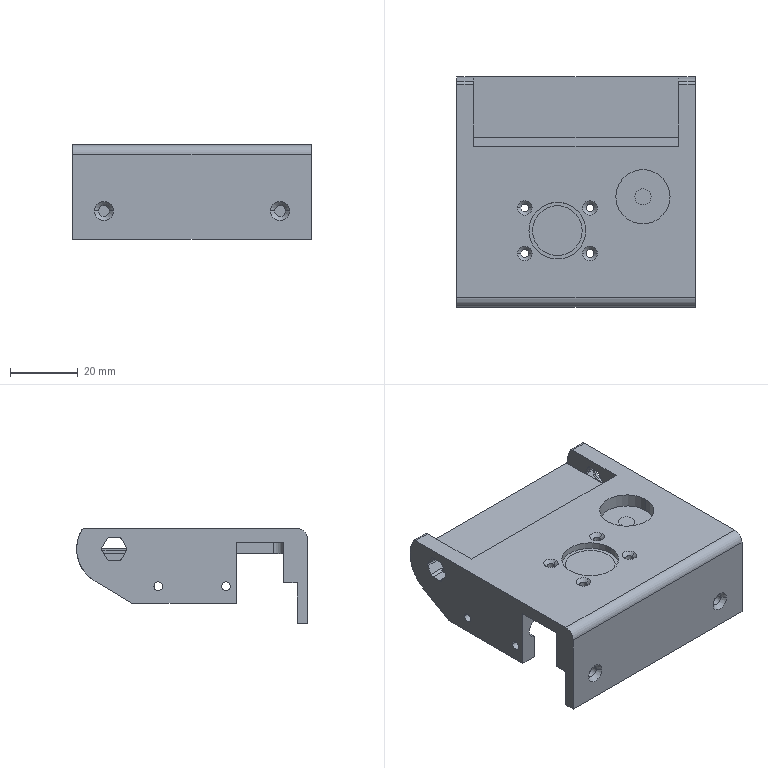NC program | NX | posted with a generic post | part box 70.5 x 68.1 x 28 mm
Lines 81 to 1012 of 7250:
(FLOOR_WALL_2 , TOOL : D10)
N160 T10 M6
N162 G54
N164 G17 G0 G90 X73.15 Y-43.397 B0. C0. S9500 M3
N166 G43 Z30. H10
N168 Z-2.85
N170 G94 G1 Z-5.85 F1000.
N172 Y-40.397
N174 Y40.397 F3000.
N176 X72.15
N178 Y-40.397
N180 X71.15
N182 Y40.397
N184 X70.15
N186 Y-40.397
N188 X69.15
N190 Y40.397
N192 X68.15
N194 Y-40.397
N196 X67.15
N198 Y40.397
N200 X66.644
N202 X66.15
N204 Y-40.397
N206 X65.776
N208 X65.15
N210 Y40.397
N212 X64.15
N214 Y-40.397
N216 X63.15
N218 Y40.397
N220 X62.15
N222 Y-40.397
N224 X61.15
N226 Y40.397
N228 X60.15
N230 Y-40.397
N232 X59.15
N234 Y40.397
N236 X58.15
N238 Y-40.397
N240 X57.15
N242 Y40.397
N244 X56.15
N246 Y-40.397
N248 X55.15
N250 Y40.397
N252 X54.15
N254 Y-40.397
N256 X53.15
N258 Y40.397
N260 X52.15
N262 Y-40.397
N264 X51.15
N266 Y40.397
N268 X50.15
N270 Y-40.397
N272 X49.15
N274 Y40.397
N276 X48.15
N278 Y-40.397
N280 X47.15
N282 Y40.397
N284 X46.15
N286 Y-40.397
N288 X45.15
N290 Y40.397
N292 X44.15
N294 Y-40.397
N296 X43.15
N298 Y40.397
N300 X42.15
N302 Y-40.397
N304 X41.15
N306 Y40.397
N308 X40.15
N310 Y-40.397
N312 X39.15
N314 Y40.397
N316 X38.15
N318 Y-40.397
N320 X37.15
N322 Y40.397
N324 X36.15
N326 Y-40.397
N328 X35.15
N330 Y40.397
N332 X34.15
N334 Y-40.397
N336 X33.15
N338 Y40.397
N340 X32.15
N342 Y-40.397
N344 X31.15
N346 Y40.397
N348 X30.15
N350 Y-40.397
N352 X29.15
N354 Y40.397
N356 X28.15
N358 Y-40.397
N360 X27.15
N362 Y40.397
N364 X26.15
N366 Y-40.397
N368 X25.15
N370 Y40.397
N372 X24.15
N374 Y-40.397
N376 X23.15
N378 Y40.397
N380 X22.15
N382 Y-40.397
N384 X21.15
N386 Y40.397
N388 X20.15
N390 Y-40.397
N392 X19.15
N394 Y40.397
N396 X18.15
N398 Y-40.397
N400 X17.15
N402 Y40.397
N404 X16.15
N406 Y-40.397
N408 X15.15
N410 Y40.397
N412 X14.15
N414 Y-40.397
N416 X13.15
N418 Y40.397
N420 X12.15
N422 Y-40.397
N424 X11.15
N426 Y40.397
N428 X10.15
N430 Y-40.397
N432 X9.15
N434 Y40.397
N436 X8.15
N438 Y-40.397
N440 Y-43.4
N442 Z-2.85
N444 G0 Z30.
(ADAPTIVE_MILLING_COPY , TOOL : D10)
N446 X14.586 Y-41.708
N448 Z-20.85
N450 G1 Z-23.85 F1000.
N452 G3 X16. Y-40.294 R2.03 F3000.
N454 X12.857 Y-39.655 R6.057
N456 X12.02 Y-40.252 R1.803
N458 G1 Y-40.377
N460 G3 X13.172 Y-41.477 R1.104
N462 G1 X14.952 Y-41.392
N464 G3 X16. Y-40.294 R1.104
N466 X12.824 Y-39.329 R3.152
N468 X12.02 Y-40.303 R1.124
N470 X13.127 Y-41.404 R1.104
N472 G1 X14.906 Y-41.394
N474 G3 X16. Y-40.294 R1.104
N476 X14.067 Y-38.886 R2.409
N478 X12.234 Y-39.414 R1.891
N480 X12.02 Y-40.244 R1.35
N482 X13.09 Y-41.345 R1.104
N484 G1 X14.87 Y-41.393
N486 G3 X16. Y-40.294 R1.104
N488 X14.831 Y-38.788 R1.871
N490 X12.354 Y-38.943 R2.282
N492 X12.02 Y-40.021 R1.337
N494 X13.03 Y-41.118 R1.106
N496 G1 X14.81 Y-41.265
N498 G3 X16. Y-40.169 R1.104
N500 X14.791 Y-38.428 R1.881
N502 X12.322 Y-38.639 R2.246
N504 X12.021 Y-39.688 R1.367
N506 X12.98 Y-40.78 R1.106
N508 G1 X14.759 Y-41.009
N510 G3 X16. Y-39.919 R1.103
N512 X14.64 Y-38.024 R1.947
N514 X12.296 Y-38.33 R2.171
N516 X12.021 Y-39.352 R1.396
N518 X12.929 Y-40.436 R1.106
N520 G1 X14.708 Y-40.752
N522 G3 X16. Y-39.669 R1.103
N524 X14.607 Y-37.672 R1.968
N526 X12.273 Y-38.022 R2.137
N528 X12.021 Y-39.01 R1.413
N530 X12.949 Y-40.098 R1.106
N532 G1 X14.728 Y-40.38
N534 G3 X16. Y-39.294 R1.103
N536 X14.686 Y-37.368 R1.939
N538 X12.33 Y-37.622 R2.228
N540 X12.022 Y-38.676 R1.359
N542 X12.9 Y-39.755 R1.106
N544 G1 X14.678 Y-40.121
N546 G3 X16. Y-39.044 R1.103
N548 X14.533 Y-36.972 R2.
N550 X12.302 Y-37.315 R2.164
N552 X12.022 Y-38.346 R1.394
N554 X12.926 Y-39.429 R1.106
N556 G1 X14.704 Y-39.751
N558 G3 X16. Y-38.669 R1.103
N560 X14.613 Y-36.666 R1.973
N562 X12.277 Y-37.01 R2.142
N564 X12.023 Y-38.004 R1.41
N566 X12.946 Y-39.091 R1.106
N568 G1 X14.724 Y-39.379
N570 G3 X16. Y-38.294 R1.103
N572 X14.691 Y-36.365 R1.939
N574 X12.334 Y-36.614 R2.227
N576 X12.023 Y-37.671 R1.355
N578 X12.972 Y-38.762 R1.106
N580 G1 X14.749 Y-39.008
N582 G3 X16. Y-37.919 R1.103
N584 X14.653 Y-36.013 R1.956
N586 X12.306 Y-36.309 R2.189
N588 X12.023 Y-37.343 R1.393
N590 X12.926 Y-38.427 R1.106
N592 G1 X14.703 Y-38.751
N594 G3 X16. Y-37.669 R1.103
N596 X14.616 Y-35.663 R1.974
N598 X12.28 Y-36.004 R2.143
N600 X12.024 Y-37.019 R1.328
N602 X12.956 Y-38.107 R1.106
N604 G1 X14.733 Y-38.381
N606 G3 X16. Y-37.294 R1.103
N608 X14.696 Y-35.359 R1.948
N610 X12.341 Y-35.61 R2.196
N612 X12.024 Y-36.594 R1.396
N614 X12.927 Y-37.678 R1.106
N616 G1 X14.703 Y-38.001
N618 G3 X16. Y-36.919 R1.103
N620 X14.52 Y-34.954 R1.997
N622 X12.398 Y-35.252 R2.083
N624 X12.052 Y-36.218 R1.725
N626 X13.01 Y-37.493 R1.104
N628 G1 X14.765 Y-37.695
N630 G3 X15.988 Y-36.52 R1.103
N632 X13.967 Y-34.496 R2.156
N634 X12.292 Y-35.092 R1.673
N636 X12.114 Y-35.848 R1.712
N638 X13.058 Y-37.06 R1.104
N640 G1 X13.951 Y-37.188
N642 X14.847 Y-37.29
N644 G3 X15.913 Y-36.025 R1.103
N646 X14.277 Y-34.228 R2.011
N648 X12.411 Y-34.625 R1.893
N650 X12.128 Y-35.639 R1.552
N652 X13.118 Y-36.795 R1.104
N654 G1 X13.98 Y-36.887
N656 X14.845 Y-36.953
N658 G3 X15.88 Y-35.794 R1.104
N660 X14.452 Y-33.961 R1.896
N662 X12.371 Y-34.362 R1.881
N664 X12.15 Y-35.235 R1.355
N666 X13.074 Y-36.321 R1.106
N668 G1 X14.585 Y-36.566
N670 G3 X15.859 Y-35.42 R1.103
N672 X14.449 Y-33.643 R1.877
N674 X12.369 Y-34.05 R1.878
N676 X12.15 Y-35.002 R1.461
N678 X13.081 Y-36.089 R1.106
N680 G1 X13.915 Y-36.225
N682 X14.753 Y-36.335
N684 G3 X15.85 Y-35.235 R1.104
N686 X14.515 Y-33.344 R1.851
N688 X12.412 Y-33.682 R1.973
N690 X12.15 Y-34.686 R1.403
N692 X13.123 Y-35.779 R1.106
N694 G1 X13.956 Y-35.881
N696 X14.792 Y-35.959
N698 G3 X15.85 Y-34.86 R1.104
N700 X14.457 Y-33.011 R1.854
N702 X12.375 Y-33.413 R1.893
N704 X12.15 Y-34.371 R1.45
N706 X13.077 Y-35.457 R1.106
N708 G1 X13.911 Y-35.597
N710 X14.749 Y-35.71
N712 G3 X15.85 Y-34.61 R1.104
N714 X14.519 Y-32.717 R1.848
N716 X12.416 Y-33.047 R1.97
N718 X12.15 Y-34.058 R1.4
N720 X13.121 Y-35.15 R1.106
N722 G1 X13.954 Y-35.254
N724 X14.789 Y-35.335
N726 G3 X15.85 Y-34.235 R1.104
N728 X14.464 Y-32.38 R1.859
N730 X12.379 Y-32.778 R1.91
N732 X12.15 Y-33.74 R1.442
N734 X13.073 Y-34.826 R1.106
N736 G1 X13.907 Y-34.969
N738 X14.745 Y-35.085
N740 G3 X15.85 Y-33.985 R1.104
N742 X14.406 Y-32.048 R1.874
N744 X12.42 Y-32.414 R1.948
N746 X12.15 Y-33.43 R1.398
N748 X13.119 Y-34.523 R1.106
N750 G1 X13.952 Y-34.628
N752 X14.788 Y-34.71
N754 G3 X15.85 Y-33.61 R1.104
N756 X14.473 Y-31.749 R1.852
N758 X12.385 Y-32.139 R1.923
N760 X12.15 Y-33.108 R1.433
N762 X13.068 Y-34.193 R1.106
N764 G1 X13.902 Y-34.34
N766 X14.741 Y-34.46
N768 G3 X15.85 Y-33.36 R1.104
N770 X14.413 Y-31.418 R1.874
N772 X12.425 Y-31.774 R1.949
N774 X12.15 Y-32.798 R1.395
N776 X13.114 Y-33.89 R1.106
N778 G1 X13.947 Y-34.
N780 X14.783 Y-34.085
N782 G3 X15.85 Y-32.985 R1.104
N784 X14.476 Y-31.121 R1.852
N786 X12.387 Y-31.503 R1.921
N788 X12.15 Y-32.461 R1.413
N790 X13.052 Y-33.543 R1.106
N792 G1 X13.887 Y-33.702
N794 X14.726 Y-33.835
N796 G3 X15.85 Y-32.735 R1.104
N798 X14.537 Y-30.829 R1.85
N800 X12.429 Y-31.135 R1.991
N802 X12.15 Y-32.165 R1.394
N804 X13.108 Y-33.256 R1.106
N806 G1 X13.942 Y-33.371
N808 X14.778 Y-33.46
N810 G3 X15.85 Y-32.36 R1.104
N812 X14.481 Y-30.493 R1.854
N814 X12.39 Y-30.867 R1.922
N816 X12.15 Y-31.826 R1.403
N818 X13.045 Y-32.907 R1.106
N820 G1 X14.545 Y-33.191
N822 G3 X15.85 Y-32.11 R1.103
N824 X14.428 Y-30.154 R1.88
N826 X12.434 Y-30.499 R1.983
N828 X12.15 Y-31.538 R1.392
N830 X13.107 Y-32.629 R1.106
N832 G1 X13.94 Y-32.744
N834 X14.776 Y-32.835
N836 G3 X15.85 Y-31.735 R1.104
N838 X14.488 Y-29.865 R1.845
N840 X12.395 Y-30.231 R1.932
N842 X12.15 Y-31.214 R1.419
N844 X13.054 Y-32.296 R1.106
N846 G1 X13.889 Y-32.454
N848 X14.728 Y-32.585
N850 G3 X15.85 Y-31.485 R1.104
N852 X14.435 Y-29.525 R1.88
N854 X12.361 Y-29.962 R1.886
N856 X12.15 Y-30.914 R1.49
N858 X13.107 Y-32.005 R1.106
N860 G1 X13.94 Y-32.12
N862 X14.777 Y-32.21
N864 G3 X15.85 Y-31.11 R1.104
N866 X14.497 Y-29.236 R1.832
N868 X12.402 Y-29.594 R1.942
N870 X12.15 Y-30.585 R1.412
N872 X13.14 Y-31.679 R1.106
N874 G1 X13.973 Y-31.768
N876 X14.807 Y-31.834
N878 G3 X15.85 Y-30.735 R1.104
N880 X14.441 Y-28.897 R1.858
N882 X12.364 Y-29.323 R1.885
N884 X12.15 Y-30.278 R1.484
N886 X13.099 Y-31.367 R1.106
N888 G1 X13.933 Y-31.489
N890 X14.77 Y-31.585
N892 G3 X15.85 Y-30.485 R1.104
N894 X14.601 Y-28.643 R1.816
N896 X12.392 Y-28.973 R1.963
N898 X12.15 Y-29.951 R1.423
N900 X13.163 Y-31.048 R1.106
N902 G1 X14.002 Y-31.12
N904 X14.844 Y-31.169
N906 G3 X15.855 Y-30.216 R1.106
N908 X14.904 Y-28.471 R1.683
N910 X12.448 Y-28.589 R2.111
N912 X12.15 Y-29.639 R1.374
N914 X13.119 Y-30.731 R1.106
N916 G1 X13.976 Y-30.84
N918 X14.837 Y-30.923
N920 G3 X15.887 Y-29.968 R1.106
N922 X14.879 Y-28.128 R1.75
N924 X12.429 Y-28.294 R2.088
N926 X12.15 Y-29.324 R1.394
N928 X13.077 Y-30.411 R1.106
N930 G1 X14.656 Y-30.662
N932 G3 X15.92 Y-29.72 R1.104
N934 X14.863 Y-27.785 R1.788
N936 X12.5 Y-27.899 R2.193
N938 X12.15 Y-28.997 R1.328
N940 X13.028 Y-30.074 R1.106
N942 G1 X14.64 Y-30.406
N944 G3 X15.952 Y-29.472 R1.104
N946 X14.847 Y-27.442 R1.833
N948 X12.487 Y-27.589 R2.184
N950 X12.15 Y-28.672 R1.334
N952 X13.064 Y-29.757 R1.106
N954 G1 X14.725 Y-30.041
N956 G3 X16.001 Y-29.1 R1.104
N958 X14.957 Y-27.164 R1.801
N960 X12.486 Y-27.265 R2.212
N962 X12.15 Y-28.347 R1.335
N964 X13.026 Y-29.424 R1.106
N966 G1 X13.958 Y-29.624
N968 X14.895 Y-29.8
N970 G3 X16.016 Y-28.986 R1.106
N972 X15.377 Y-27.097 R1.668
N974 X12.488 Y-26.934 R2.312
N976 X12.15 Y-28.018 R1.334
N978 X13.002 Y-29.09 R1.106
N980 G1 X14.788 Y-29.503
N982 G3 X16.052 Y-28.853 R1.106
N984 X15.607 Y-26.927 R1.622
N986 X12.521 Y-26.573 R2.403
N988 X12.15 Y-27.697 R1.323
N990 X12.966 Y-28.76 R1.108
N992 G1 X14.847 Y-29.263
N994 G3 X16.148 Y-28.622 R1.106
N996 X15.667 Y-26.587 R1.705
N998 X12.567 Y-26.197 R2.494
N1000 X12.15 Y-27.35 R1.288
N1002 X12.921 Y-28.399 R1.108
N1004 G1 X14.898 Y-29.019
N1006 G3 X16.243 Y-28.391 R1.106
N1008 X15.825 Y-26.335 R1.746
N1010 X12.625 Y-25.81 R2.605
N1012 X12.15 Y-27.018 R1.276
N1014 X12.889 Y-28.057 R1.108
N1016 G1 X14.962 Y-28.778
N1018 G3 X16.339 Y-28.16 R1.104
N1020 X15.909 Y-25.992 R1.816
N1022 X12.596 Y-25.484 R2.651
N1024 X12.15 Y-26.662 R1.278
N1026 X12.906 Y-27.707 R1.108
N1028 G1 X15.122 Y-28.437
N1030 G3 X16.483 Y-27.813 R1.106
N1032 X16.198 Y-25.876 R1.743
N1034 X12.616 Y-25.113 R2.768
N1036 X12.15 Y-26.31 R1.276
N1038 X12.859 Y-27.338 R1.108
N1040 G1 X15.169 Y-28.217
N1042 G3 X16.513 Y-27.739 R1.106
N1044 X16.517 Y-25.846 R1.647
N1046 X12.72 Y-24.685 R2.89
N1048 X12.15 Y-25.952 R1.256
N1050 X12.836 Y-26.971 R1.108
N1052 G1 X15.296 Y-27.969
N1054 G3 X16.582 Y-27.62 R1.108
N1056 X16.728 Y-25.641 R1.666
N1058 X12.768 Y-24.286 R3.016
N1060 X12.15 Y-25.698 R1.362
N1062 X12.838 Y-26.718 R1.108
N1064 G1 X15.45 Y-27.772
N1066 G3 X16.735 Y-27.421 R1.108
N1068 X16.894 Y-25.326 R1.768
N1070 X12.726 Y-23.931 R3.115
N1072 X12.15 Y-25.204 R1.259
N1074 X12.807 Y-26.211 R1.111
N1076 G1 X15.647 Y-27.461
N1078 G3 X16.963 Y-27.124 R1.107
N1080 X17.075 Y-25.013 R1.848
N1082 X12.809 Y-23.495 R3.266
N1084 X12.15 Y-24.938 R1.37
N1086 X12.806 Y-25.944 R1.111
N1088 G1 X15.799 Y-27.263
N1090 G3 X17.115 Y-26.926 R1.106
N1092 X17.294 Y-24.743 R1.923
N1094 X12.847 Y-23.081 R3.405
N1096 X12.15 Y-24.551 R1.376
N1098 X12.836 Y-25.57 R1.108
N1100 G1 X16.124 Y-26.905
N1102 G3 X17.316 Y-26.664 R1.108
N1104 X17.639 Y-24.784 R1.779
N1106 X12.972 Y-22.613 R3.57
N1108 X12.15 Y-24.138 R1.377
N1110 X12.803 Y-25.143 R1.111
N1112 G1 X16.297 Y-26.698
N1114 G3 X17.414 Y-26.566 R1.112
N1116 X17.958 Y-24.874 R1.664
N1118 X12.926 Y-22.216 R3.692
N1120 X12.15 Y-23.726 R1.382
N1122 X12.738 Y-24.699 R1.112
N1124 G1 X16.331 Y-26.591
N1126 G3 X17.513 Y-26.49 R1.111
N1128 X18.191 Y-24.49 R1.838
N1130 X12.915 Y-21.789 R3.872
N1132 X12.15 Y-23.296 R1.389
N1134 X12.704 Y-24.251 R1.112
N1136 G1 X16.495 Y-26.42
N1138 G3 X17.711 Y-26.338 R1.108
N1140 X18.487 Y-24.365 R1.891
N1142 X13.049 Y-21.286 R4.079
N1144 X12.15 Y-22.868 R1.414
N1146 X12.699 Y-23.819 R1.112
N1148 G1 X16.788 Y-26.189
N1150 G3 X18.009 Y-26.109 R1.108
N1152 X18.775 Y-24.122 R1.976
N1154 X13.096 Y-20.812 R4.284
N1156 X12.15 Y-22.411 R1.423
N1158 X12.668 Y-23.345 R1.113
N1160 G1 X16.955 Y-26.018
N1162 G3 X18.207 Y-25.957 R1.108
N1164 X19.081 Y-23.934 R2.035
N1166 X15.181 Y-20.104 R4.486
N1168 X12.473 Y-20.761 R3.339
N1170 X12.15 Y-21.955 R1.507
N1172 X12.657 Y-22.882 R1.113
N1174 G1 X17.227 Y-25.806
N1176 G3 X18.37 Y-25.832 R1.112
N1178 X19.402 Y-24.094 R1.866
N1180 X16.84 Y-20.106 R4.432
N1182 X12.874 Y-19.997 R4.281
N1184 X12.15 Y-21.49 R1.408
N1186 X12.634 Y-22.402 R1.115
N1188 G1 X17.452 Y-25.658
N1190 G3 X18.489 Y-25.763 R1.115
N1192 X19.703 Y-24.167 R1.811
N1194 X17.668 Y-20.003 R4.446
N1196 X13.043 Y-19.423 R4.702
N1198 X12.15 Y-21.021 R1.444
N1200 X12.623 Y-21.925 R1.116
N1202 G1 X17.788 Y-25.507
N1204 G3 X18.836 Y-25.62 R1.113
N1206 X20.047 Y-24.004 R1.93
N1208 X18.185 Y-19.742 R4.61
N1210 X13.135 Y-18.884 R5.003
N1212 X12.15 Y-20.527 R1.473
N1214 X12.597 Y-21.412 R1.116
N1216 G1 X17.993 Y-25.393
N1218 G3 X19.067 Y-25.524 R1.112
N1220 X20.422 Y-23.731 R2.078
N1222 X18.436 Y-19.26 R4.881
N1224 X13.264 Y-18.32 R5.295
N1226 X12.15 Y-19.535 R1.582
N1228 G1 Y-20.035
N1230 G3 X12.588 Y-20.913 R1.116
N1232 G1 X18.33 Y-25.243
N1234 G3 X19.413 Y-25.381 R1.112
N1236 X20.782 Y-23.638 R2.137
N1238 X19.13 Y-19.139 R4.974
N1240 X13.469 Y-17.721 R5.693
N1242 X12.227 Y-18.698 R2.008
N1244 X12.15 Y-19.643 R2.957
N1246 X12.586 Y-20.519 R1.116
N1248 G1 X18.654 Y-25.116
N1250 G3 X19.603 Y-25.302 R1.116
N1252 X21.056 Y-23.88 R1.957
N1254 X20.037 Y-19.317 R4.878
N1256 X13.796 Y-17.083 R6.142
N1258 X12.267 Y-18.086 R2.454
N1260 X12.15 Y-19.116 R2.365
N1262 X12.564 Y-19.976 R1.117
N1264 G1 X18.907 Y-25.036
N1266 G3 X19.736 Y-25.266 R1.128
N1268 X21.335 Y-24.037 R1.915
N1270 X20.837 Y-19.503 R4.832
N1272 X13.957 Y-16.494 R6.516
N1274 X12.289 Y-17.512 R2.715
N1276 X12.15 Y-18.595 R2.219
N1278 X12.542 Y-19.437 R1.117
N1280 G1 X19.132 Y-24.985
N1282 G3 X19.984 Y-25.234 R1.127
N1284 X21.773 Y-23.871 R2.087
N1286 X21.3 Y-19.204 R5.095
N1288 X14.042 Y-15.912 R6.861
N1290 X12.275 Y-16.998 R2.775
N1292 X12.15 Y-18.047 R2.299
N1294 X12.529 Y-18.877 R1.118
N1296 G1 X19.491 Y-24.925
N1298 G3 X20.356 Y-25.185 R1.118
N1300 X22.167 Y-23.836 R2.175
N1302 X21.907 Y-19.141 R5.247
N1304 X14.29 Y-15.285 R7.254
N1306 X12.345 Y-16.328 R3.361
N1308 X12.15 Y-17.497 R1.956
N1310 X12.517 Y-18.317 R1.118
N1312 G1 X19.851 Y-24.866
N1314 G3 X20.728 Y-25.136 R1.117
N1316 X22.594 Y-23.762 R2.256
N1318 X22.443 Y-18.936 R5.485
N1320 X14.398 Y-14.682 R7.607
N1322 X12.341 Y-15.772 R3.498
N1324 X12.15 Y-16.934 R1.965
N1326 X12.511 Y-17.749 R1.118
N1328 G1 X13.164 Y-18.342
N1330 X14.645 Y-19.686 Z-23.75
N1332 X18.398 Y-23.092
N1334 X19.879 Y-24.436 Z-23.85
N1336 X20.423 Y-24.914
N1338 G3 X21.035 Y-25.1 R1.15
N1340 X22.867 Y-23.983 R2.123
N1342 X23.165 Y-19.167 R5.428
N1344 X14.618 Y-14.047 R8.007
N1346 X12.331 Y-15.213 R3.637
N1348 X12.15 Y-16.357 R1.995
N1350 X12.492 Y-17.154 R1.127
N1352 G1 X13.196 Y-17.824
N1354 X14.646 Y-19.203 Z-23.75
N1356 X18.631 Y-22.994
N1358 X20.08 Y-24.372 Z-23.85
N1360 X20.656 Y-24.903
N1362 G3 X21.285 Y-25.1 R1.148
N1364 X23.268 Y-24.01 R2.215
N1366 X23.824 Y-19.325 R5.512
N1368 X14.763 Y-13.416 R8.404
N1370 X12.347 Y-14.603 R3.894
N1372 X12.15 Y-15.776 R1.952
N1374 X12.481 Y-16.563 R1.128
N1376 G1 X13.216 Y-17.281
N1378 X14.646 Y-18.68 Z-23.75
N1380 X18.947 Y-22.886
N1382 X20.377 Y-24.284 Z-23.85
N1384 X21.021 Y-24.896
N1386 G3 X21.66 Y-25.1 R1.146
N1388 X23.746 Y-23.949 R2.341
N1390 X24.378 Y-19.146 R5.748
N1392 X14.945 Y-12.772 R8.818
N1394 X12.387 Y-13.957 R4.237
N1396 X12.15 Y-15.178 R1.835
N1398 X12.471 Y-15.955 R1.128
N1400 G1 X13.235 Y-16.722
N1402 X14.646 Y-18.139 Z-23.75
N1404 X19.302 Y-22.815
N1406 X20.714 Y-24.232 Z-23.85
N1408 X21.044 Y-24.566
N1410 X21.387 Y-24.889
N1412 G3 X22.035 Y-25.1 R1.145
N1414 X24.158 Y-24.004 R2.415
N1416 X25.008 Y-19.228 R5.88
N1418 X15.041 Y-12.131 R9.232
N1420 X12.374 Y-13.369 R4.314
N1422 X12.15 Y-14.576 R1.867
N1424 X12.461 Y-15.343 R1.129
N1426 G1 X13.252 Y-16.157
N1428 X14.646 Y-17.591 Z-23.75
N1430 X19.672 Y-22.762
N1432 X21.066 Y-24.196 Z-23.85
N1434 X21.403 Y-24.546
N1436 X21.753 Y-24.883
N1438 G3 X22.41 Y-25.1 R1.144
N1440 X24.651 Y-23.972 R2.531
N1442 X25.566 Y-18.961 R6.187
N1444 X15.292 Y-11.46 R9.699
N1446 X12.382 Y-12.749 R4.591
N1448 X12.15 Y-13.965 R1.846
N1450 X12.453 Y-14.723 R1.13
N1452 G1 X13.269 Y-15.582
N1454 X14.647 Y-17.032 Z-23.75
N1456 X20.04 Y-22.708
N1458 X21.418 Y-24.158 Z-23.85
N1460 X21.762 Y-24.524
N1462 X22.12 Y-24.877
N1464 G3 X22.785 Y-25.1 R1.143
N1466 X25.147 Y-23.951 R2.625
N1468 X26.163 Y-18.833 R6.402
N1470 X15.454 Y-10.792 R10.153
N1472 X12.413 Y-12.093 R4.879
N1474 X12.15 Y-13.349 R1.787
N1476 X12.449 Y-14.104 R1.13
N1478 G1 X13.275 Y-14.98
N1480 X14.647 Y-16.436 Z-23.75
N1482 X20.495 Y-22.643
N1484 X21.866 Y-24.098 Z-23.85
N1486 X22.234 Y-24.494
N1488 X22.617 Y-24.874
N1490 G3 X23.285 Y-25.1 R1.143
N1492 X25.648 Y-23.943 R2.687
N1494 X26.795 Y-18.844 R6.591
N1496 X15.775 Y-10.103 R10.627
N1498 X12.468 Y-11.404 R5.284
N1500 X12.15 Y-12.093 R1.354
N1502 G1 Y-12.843
N1504 G3 X12.45 Y-13.598 R1.13
N1506 G1 X13.274 Y-14.47
N1508 X14.647 Y-15.924 Z-23.75
N1510 X20.952 Y-22.602
N1512 X22.325 Y-24.056 Z-23.85
N1514 X22.713 Y-24.473
N1516 X23.118 Y-24.875
N1518 G3 X23.785 Y-25.1 R1.143
N1520 X26.159 Y-23.95 R2.759
N1522 X27.415 Y-18.747 R6.815
N1524 X20.52 Y-10.188 R11.067
N1526 X13.929 Y-9.858 R9.176
N1528 X12.249 Y-11.088 R3.057
N1530 X12.15 Y-12.207 R2.948
N1532 X12.443 Y-12.954 R1.13
N1534 G1 X13.289 Y-13.869
N1536 X14.647 Y-15.337 Z-23.75
N1538 X21.367 Y-22.601
N1540 X22.725 Y-24.069 Z-23.85
N1542 X23.098 Y-24.477
N1544 X23.486 Y-24.869
N1546 G3 X24.16 Y-25.1 R1.142
N1548 X26.749 Y-23.864 R2.91
N1550 X28.028 Y-18.536 R7.12
N1552 X21.457 Y-9.817 R11.493
N1554 X14.288 Y-9.076 R9.931
N1556 X12.312 Y-10.322 R3.887
N1558 X12.15 Y-11.56 R2.366
N1560 X12.439 Y-12.304 R1.131
N1562 G1 X13.295 Y-13.237
N1564 X14.647 Y-14.711 Z-23.75
N1566 X21.884 Y-22.601
N1568 X23.236 Y-24.075 Z-23.85
N1570 X23.601 Y-24.478
N1572 X23.983 Y-24.867
N1574 G3 X24.66 Y-25.1 R1.142
N1576 X27.345 Y-23.792 R3.004
N1578 X28.638 Y-18.216 R7.457
N1580 X22.295 Y-9.423 R11.992
N1582 X14.68 Y-8.292 R10.67
N1584 X12.335 Y-9.636 R4.34
N1586 X12.15 Y-10.912 R2.257
N1588 X12.436 Y-11.652 R1.131
N1590 G1 X13.301 Y-12.602
N1592 X14.647 Y-14.081 Z-23.75
N1594 X22.399 Y-22.601
N1596 X23.745 Y-24.08 Z-23.85
N1598 X24.456 Y-24.846
N1600 G3 X25.16 Y-25.1 R1.134
N1602 X27.865 Y-23.825 R3.054
N1604 X29.306 Y-18.28 R7.579
N1606 X23.675 Y-9.387 R12.325
N1608 X15.226 Y-7.484 R11.615
N1610 X12.375 Y-8.922 R5.002
N1612 X12.15 Y-9.504 R1.874
N1614 G1 Y-10.254
N1616 G3 X12.437 Y-10.995 R1.131
N1618 G1 X13.299 Y-11.941
N1620 X14.647 Y-13.419 Z-23.75
N1622 X23.02 Y-22.601
N1624 X24.368 Y-24.078 Z-23.85
N1626 X24.729 Y-24.48
N1628 X25.106 Y-24.866
N1630 G3 X25.785 Y-25.1 R1.142
N1632 X28.389 Y-23.867 R3.052
N1634 X29.974 Y-18.357 R7.71
N1636 X24.823 Y-9.286 R12.696
N1638 X15.8 Y-6.696 R12.414
N1640 X12.519 Y-8.094 R5.852
N1642 X12.15 Y-8.848 R1.304
N1644 G1 Y-9.598
N1646 G3 X12.434 Y-10.336 R1.131
N1648 G1 X13.305 Y-11.298
N1650 X14.647 Y-12.781 Z-23.75
N1652 X23.534 Y-22.6
N1654 X24.877 Y-24.083 Z-23.85
N1656 X25.58 Y-24.844
N1658 G3 X26.285 Y-25.1 R1.134
N1660 X28.914 Y-23.914 R3.094
N1662 X30.641 Y-18.444 R7.797
N1664 X25.572 Y-8.915 R13.075
N1666 X16.03 Y-5.963 R13.017
N1668 X12.511 Y-7.424 R6.084
N1670 X12.15 Y-8.166 R1.306
N1672 G1 Y-8.916
N1674 G3 X12.431 Y-9.651 R1.131
N1676 G1 X13.311 Y-10.632
N1678 X14.647 Y-12.12 Z-23.75
N1680 X24.051 Y-22.6
N1682 X25.387 Y-24.089 Z-23.85
N1684 X26.077 Y-24.842
N1686 G3 X26.785 Y-25.1 R1.134
N1688 X29.525 Y-23.877 R3.177
N1690 X31.304 Y-18.293 R8.022
N1692 X26.426 Y-8.643 R13.484
N1694 X16.531 Y-5.197 R13.72
N1696 X12.704 Y-6.564 R6.933
N1698 X12.15 Y-7.495 R1.398
N1700 G1 Y-8.245
N1702 G3 X12.432 Y-8.98 R1.131
N1704 G1 X13.31 Y-9.958
N1706 X14.647 Y-11.445 Z-23.75
N1708 X24.673 Y-22.6
N1710 X26.01 Y-24.088 Z-23.85
N1712 X26.702 Y-24.842
N1714 G3 X27.41 Y-25.1 R1.134
N1716 X30.141 Y-23.847 R3.237
N1718 X31.978 Y-18.275 R8.212
N1720 X27.651 Y-8.729 R13.813
N1722 X17.055 Y-4.44 R14.472
N1724 X12.826 Y-5.773 R7.604
N1726 X12.15 Y-6.798 R1.554
N1728 G1 Y-7.548
N1730 G3 X12.429 Y-8.28 R1.132
N1732 G1 X13.317 Y-9.276
N1734 X14.647 Y-10.769 Z-23.75
N1736 X25.189 Y-22.6
N1738 X26.52 Y-24.093 Z-23.85
N1740 X27.199 Y-24.84
N1742 G3 X27.91 Y-25.1 R1.133
N1744 X30.759 Y-23.824 R3.316
N1746 X32.658 Y-18.266 R8.404
N1748 X28.596 Y-8.588 R14.217
N1750 X17.476 Y-3.691 R15.169
N1752 X12.87 Y-5.044 R8.069
N1754 X12.15 Y-6.101 R1.574
N1756 G1 Y-6.851
N1758 G3 X12.429 Y-7.583 R1.132
N1760 G1 X13.316 Y-8.579
N1762 X14.647 Y-10.072 Z-23.75
N1764 X25.813 Y-22.6
N1766 X27.144 Y-24.093 Z-23.85
N1768 X27.824 Y-24.84
N1770 G3 X28.535 Y-25.1 R1.133
N1772 X31.296 Y-23.898 R3.326
N1774 X33.342 Y-18.265 R8.499
N1776 X29.784 Y-8.752 R14.562
N1778 X18.165 Y-2.947 R15.956
N1780 X13.132 Y-4.155 R9.012
N1782 X12.153 Y-5.385 R1.879
N1784 G1 X12.15 Y-5.403
N1786 Y-6.153
N1788 G3 X12.426 Y-6.882 R1.132
N1790 G1 X13.322 Y-7.895
N1792 X14.647 Y-9.393 Z-23.75
N1794 X26.328 Y-22.6
N1796 X27.653 Y-24.098 Z-23.85
N1798 X28.322 Y-24.837
N1800 G3 X29.035 Y-25.1 R1.133
N1802 X32.004 Y-23.795 R3.467
N1804 X34.037 Y-18.023 R8.83
N1806 X30.073 Y-7.895 R15.134
N1808 X18.125 Y-2.194 R16.411
N1810 X13.106 Y-3.464 R9.09
N1812 X12.15 Y-4.71 R1.839
N1814 G1 Y-5.46
N1816 G3 X12.426 Y-6.189 R1.132
N1818 G1 X13.322 Y-7.201
N1820 X14.647 Y-8.698 Z-23.75
N1822 X26.951 Y-22.6
N1824 X28.277 Y-24.097 Z-23.85
N1826 X28.947 Y-24.838
N1828 G3 X29.66 Y-25.1 R1.133
N1830 X32.543 Y-23.883 R3.432
N1832 X34.714 Y-18.416 R8.722
N1834 X31.421 Y-8.291 R15.252
N1836 X18.732 Y-1.448 R17.183
N1838 X13.308 Y-2.617 R9.875
N1840 X12.197 Y-3.759 R2.422
N1842 X12.15 Y-4.75 R5.766
N1844 X12.426 Y-5.479 R1.132
N1846 G1 X13.322 Y-6.491
N1848 X14.647 Y-7.989 Z-23.75
N1850 X27.577 Y-22.599
N1852 X28.902 Y-24.097 Z-23.85
N1854 X29.572 Y-24.838
N1856 G3 X30.285 Y-25.1 R1.133
N1858 X33.173 Y-23.886 R3.478
N1860 X35.415 Y-18.314 R8.939
N1862 X32.286 Y-8.126 R15.679
N1864 X18.979 Y-0.688 R17.831
N1866 X13.311 Y-1.892 R10.189
N1868 X12.198 Y-3.033 R2.444
N1870 X12.15 Y-4.028 R5.377
N1872 X12.426 Y-4.757 R1.132
N1874 G1 X13.322 Y-5.771
N1876 X14.647 Y-7.269 Z-23.75
N1878 X28.203 Y-22.599
N1880 X29.528 Y-24.098 Z-23.85
N1882 X30.196 Y-24.837
N1884 G3 X30.91 Y-25.1 R1.133
N1886 X33.803 Y-23.892 R3.517
N1888 X36.102 Y-18.47 R8.982
N1890 X33.295 Y-8.181 R15.944
N1892 X19.368 Y0.067 R18.507
N1894 X13.438 Y-1.09 R10.732
N1896 X12.206 Y-2.287 R2.668
N1898 X12.15 Y-3.296 R4.205
N1900 X12.426 Y-4.024 R1.132
N1902 G1 X13.323 Y-5.04
N1904 X14.647 Y-6.54 Z-23.75
N1906 X28.83 Y-22.599
N1908 X30.154 Y-24.098 Z-23.85
N1910 X30.821 Y-24.837
N1912 G3 X31.535 Y-25.1 R1.133
N1914 X34.436 Y-23.904 R3.549
N1916 X36.784 Y-18.632 R9.023
N1918 X34.359 Y-8.362 R16.134
N1920 X19.897 Y0.814 R19.213
N1922 X13.687 Y-0.214 R11.551
N1924 X12.219 Y-1.52 R3.091
N1926 X12.15 Y-2.564 R3.569
N1928 X12.425 Y-3.292 R1.132
N1930 G1 X13.324 Y-4.311
N1932 X14.647 Y-5.811 Z-23.75
N1934 X29.457 Y-22.599
N1936 X30.78 Y-24.099 Z-23.85
N1938 X31.446 Y-24.837
N1940 G3 X32.16 Y-25.1 R1.133
N1942 X35.158 Y-23.834 R3.634
N1944 X37.531 Y-18.305 R9.394
N1946 X34.893 Y-7.708 R16.667
N1948 X20.067 Y1.589 R19.797
N1950 X13.732 Y0.552 R11.86
N1952 X12.239 Y-0.733 R3.363
N1954 X12.15 Y-1.84 R3.19
N1956 X12.425 Y-2.567 R1.132
N1958 G1 X13.325 Y-3.588
N1960 X14.647 Y-5.088 Z-23.75
N1962 X30.083 Y-22.599
N1964 X31.406 Y-24.099 Z-23.85
N1966 X32.07 Y-24.836
N1968 G3 X32.785 Y-25.1 R1.133
N1970 X35.794 Y-23.854 R3.66
N1972 X38.239 Y-18.353 R9.516
N1974 X35.957 Y-7.91 R16.961
N1976 X20.624 Y2.337 R20.521
N1978 X13.901 Y1.384 R12.566
N1980 X12.266 Y0.071 R3.887
N1982 X12.15 Y-1.208 R3.102
N1984 X12.426 Y-1.937 R1.132
N1986 G1 X13.322 Y-2.95
N1988 X14.647 Y-4.448 Z-23.75
N1990 X30.702 Y-22.599
N1992 X32.027 Y-24.097 Z-23.85
N1994 X32.697 Y-24.837
N1996 G3 X33.41 Y-25.1 R1.133
N1998 X36.431 Y-23.879 R3.685
N2000 X38.85 Y-18.974 R9.308
N2002 X38.789 Y-13.851 R68.172
N2004 X34.276 Y-4.128 R18.481
N2006 X20.216 Y3.174 R20.863
N2008 X13.764 Y2.065 R12.36
N2010 X12.256 Y0.791 R3.666